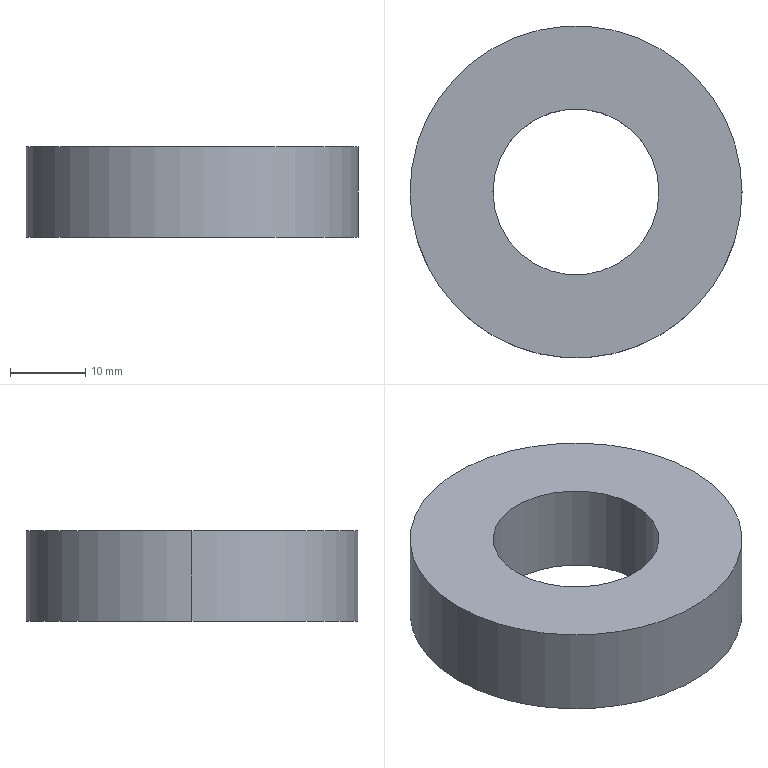Part | STEP file | 6022ZZ deep groove ball bearing MISUMI 62 | 1 solid | 6 faces | box 44 x 44 x 12 mm | volume 13685 mm3 | cylinder 4 | plane 2 | commonest cylinder face diameters 22 x2 44 x2
STEP:
#1=CARTESIAN_POINT('',(-11.,0.,6.));
#2=VERTEX_POINT('',#1);
#3=CARTESIAN_POINT('',(11.,0.,6.));
#4=VERTEX_POINT('',#3);
#5=CARTESIAN_POINT('',(0.,0.,6.));
#6=DIRECTION('',(0.,0.,1.));
#7=DIRECTION('',(1.,0.,0.));
#8=AXIS2_PLACEMENT_3D('',#5,#6,#7);
#9=CIRCLE('',#8,11.);
#10=EDGE_CURVE('',#2,#4,#9,.T.);
#11=ORIENTED_EDGE('',*,*,#10,.T.);
#12=CARTESIAN_POINT('',(11.,0.,-6.));
#13=VERTEX_POINT('',#12);
#14=CARTESIAN_POINT('',(11.,0.,6.));
#15=DIRECTION('',(0.,0.,-1.));
#16=VECTOR('',#15,1000.);
#17=LINE('',#14,#16);
#18=EDGE_CURVE('',#4,#13,#17,.T.);
#19=ORIENTED_EDGE('',*,*,#18,.T.);
#20=CARTESIAN_POINT('',(-11.,0.,-6.));
#21=VERTEX_POINT('',#20);
#22=CARTESIAN_POINT('',(0.,0.,-6.));
#23=DIRECTION('',(0.,0.,1.));
#24=DIRECTION('',(1.,0.,0.));
#25=AXIS2_PLACEMENT_3D('',#22,#23,#24);
#26=CIRCLE('',#25,11.);
#27=EDGE_CURVE('',#21,#13,#26,.T.);
#28=ORIENTED_EDGE('',*,*,#27,.F.);
#29=CARTESIAN_POINT('',(-11.,0.,6.));
#30=DIRECTION('',(0.,0.,-1.));
#31=VECTOR('',#30,1000.);
#32=LINE('',#29,#31);
#33=EDGE_CURVE('',#2,#21,#32,.T.);
#34=ORIENTED_EDGE('',*,*,#33,.F.);
#35=EDGE_LOOP('',(#11,#19,#28,#34));
#36=FACE_OUTER_BOUND('',#35,.T.);
#37=CARTESIAN_POINT('',(0.,0.,6.));
#38=DIRECTION('',(0.,0.,-1.));
#39=DIRECTION('',(-1.,0.,0.));
#40=AXIS2_PLACEMENT_3D('',#37,#38,#39);
#41=CYLINDRICAL_SURFACE('',#40,11.);
#42=ADVANCED_FACE('',(#36),#41,.F.);
#43=CARTESIAN_POINT('',(22.,0.,6.));
#44=VERTEX_POINT('',#43);
#45=CARTESIAN_POINT('',(-22.,0.,6.));
#46=VERTEX_POINT('',#45);
#47=CARTESIAN_POINT('',(0.,0.,6.));
#48=DIRECTION('',(0.,0.,1.));
#49=DIRECTION('',(1.,0.,0.));
#50=AXIS2_PLACEMENT_3D('',#47,#48,#49);
#51=CIRCLE('',#50,22.);
#52=EDGE_CURVE('',#44,#46,#51,.T.);
#53=ORIENTED_EDGE('',*,*,#52,.F.);
#54=CARTESIAN_POINT('',(22.,0.,-6.));
#55=VERTEX_POINT('',#54);
#56=CARTESIAN_POINT('',(22.,0.,6.));
#57=DIRECTION('',(0.,0.,-1.));
#58=VECTOR('',#57,1000.);
#59=LINE('',#56,#58);
#60=EDGE_CURVE('',#44,#55,#59,.T.);
#61=ORIENTED_EDGE('',*,*,#60,.T.);
#62=CARTESIAN_POINT('',(-22.,0.,-6.));
#63=VERTEX_POINT('',#62);
#64=CARTESIAN_POINT('',(0.,0.,-6.));
#65=DIRECTION('',(0.,0.,1.));
#66=DIRECTION('',(1.,0.,0.));
#67=AXIS2_PLACEMENT_3D('',#64,#65,#66);
#68=CIRCLE('',#67,22.);
#69=EDGE_CURVE('',#55,#63,#68,.T.);
#70=ORIENTED_EDGE('',*,*,#69,.T.);
#71=CARTESIAN_POINT('',(-22.,0.,6.));
#72=DIRECTION('',(0.,0.,-1.));
#73=VECTOR('',#72,1000.);
#74=LINE('',#71,#73);
#75=EDGE_CURVE('',#46,#63,#74,.T.);
#76=ORIENTED_EDGE('',*,*,#75,.F.);
#77=EDGE_LOOP('',(#53,#61,#70,#76));
#78=FACE_OUTER_BOUND('',#77,.T.);
#79=CARTESIAN_POINT('',(0.,0.,6.));
#80=DIRECTION('',(0.,0.,-1.));
#81=DIRECTION('',(-1.,0.,0.));
#82=AXIS2_PLACEMENT_3D('',#79,#80,#81);
#83=CYLINDRICAL_SURFACE('',#82,22.);
#84=ADVANCED_FACE('',(#78),#83,.T.);
#85=CARTESIAN_POINT('',(0.,0.,6.));
#86=DIRECTION('',(0.,0.,1.));
#87=DIRECTION('',(1.,0.,0.));
#88=AXIS2_PLACEMENT_3D('',#85,#86,#87);
#89=CIRCLE('',#88,22.);
#90=EDGE_CURVE('',#46,#44,#89,.T.);
#91=ORIENTED_EDGE('',*,*,#90,.T.);
#92=ORIENTED_EDGE('',*,*,#52,.T.);
#93=EDGE_LOOP('',(#91,#92));
#94=FACE_OUTER_BOUND('',#93,.T.);
#95=ORIENTED_EDGE('',*,*,#10,.F.);
#96=CARTESIAN_POINT('',(0.,0.,6.));
#97=DIRECTION('',(0.,0.,1.));
#98=DIRECTION('',(1.,0.,0.));
#99=AXIS2_PLACEMENT_3D('',#96,#97,#98);
#100=CIRCLE('',#99,11.);
#101=EDGE_CURVE('',#4,#2,#100,.T.);
#102=ORIENTED_EDGE('',*,*,#101,.F.);
#103=EDGE_LOOP('',(#95,#102));
#104=FACE_BOUND('',#103,.T.);
#105=CARTESIAN_POINT('',(0.,0.,6.));
#106=DIRECTION('',(0.,0.,1.));
#107=DIRECTION('',(1.,0.,0.));
#108=AXIS2_PLACEMENT_3D('',#105,#106,#107);
#109=PLANE('',#108);
#110=ADVANCED_FACE('',(#94,#104),#109,.T.);
#111=CARTESIAN_POINT('',(0.,0.,-6.));
#112=DIRECTION('',(0.,0.,1.));
#113=DIRECTION('',(1.,0.,0.));
#114=AXIS2_PLACEMENT_3D('',#111,#112,#113);
#115=CIRCLE('',#114,22.);
#116=EDGE_CURVE('',#63,#55,#115,.T.);
#117=ORIENTED_EDGE('',*,*,#116,.F.);
#118=ORIENTED_EDGE('',*,*,#69,.F.);
#119=EDGE_LOOP('',(#117,#118));
#120=FACE_OUTER_BOUND('',#119,.T.);
#121=ORIENTED_EDGE('',*,*,#27,.T.);
#122=CARTESIAN_POINT('',(0.,0.,-6.));
#123=DIRECTION('',(0.,0.,1.));
#124=DIRECTION('',(1.,0.,0.));
#125=AXIS2_PLACEMENT_3D('',#122,#123,#124);
#126=CIRCLE('',#125,11.);
#127=EDGE_CURVE('',#13,#21,#126,.T.);
#128=ORIENTED_EDGE('',*,*,#127,.T.);
#129=EDGE_LOOP('',(#121,#128));
#130=FACE_BOUND('',#129,.T.);
#131=CARTESIAN_POINT('',(0.,0.,-6.));
#132=DIRECTION('',(0.,0.,1.));
#133=DIRECTION('',(1.,0.,0.));
#134=AXIS2_PLACEMENT_3D('',#131,#132,#133);
#135=PLANE('',#134);
#136=ADVANCED_FACE('',(#120,#130),#135,.F.);
#137=ORIENTED_EDGE('',*,*,#60,.F.);
#138=ORIENTED_EDGE('',*,*,#90,.F.);
#139=ORIENTED_EDGE('',*,*,#75,.T.);
#140=ORIENTED_EDGE('',*,*,#116,.T.);
#141=EDGE_LOOP('',(#137,#138,#139,#140));
#142=FACE_OUTER_BOUND('',#141,.T.);
#143=CARTESIAN_POINT('',(0.,0.,6.));
#144=DIRECTION('',(0.,0.,-1.));
#145=DIRECTION('',(-1.,0.,0.));
#146=AXIS2_PLACEMENT_3D('',#143,#144,#145);
#147=CYLINDRICAL_SURFACE('',#146,22.);
#148=ADVANCED_FACE('',(#142),#147,.T.);
#149=ORIENTED_EDGE('',*,*,#18,.F.);
#150=ORIENTED_EDGE('',*,*,#101,.T.);
#151=ORIENTED_EDGE('',*,*,#33,.T.);
#152=ORIENTED_EDGE('',*,*,#127,.F.);
#153=EDGE_LOOP('',(#149,#150,#151,#152));
#154=FACE_OUTER_BOUND('',#153,.T.);
#155=CARTESIAN_POINT('',(0.,0.,6.));
#156=DIRECTION('',(0.,0.,-1.));
#157=DIRECTION('',(-1.,0.,0.));
#158=AXIS2_PLACEMENT_3D('',#155,#156,#157);
#159=CYLINDRICAL_SURFACE('',#158,11.);
#160=ADVANCED_FACE('',(#154),#159,.F.);
#161=CLOSED_SHELL('',(#42,#84,#110,#136,#148,#160));
#162=MANIFOLD_SOLID_BREP('',#161);
#163=CARTESIAN_POINT('',(0.,0.,0.));
#164=DIRECTION('',(0.,0.,1.));
#165=DIRECTION('',(1.,0.,0.));
#166=AXIS2_PLACEMENT_3D('',#163,#164,#165);
#167=(LENGTH_UNIT()NAMED_UNIT(*)SI_UNIT(.MILLI.,.METRE.));
#168=UNCERTAINTY_MEASURE_WITH_UNIT(LENGTH_MEASURE(0.00001),#167,'','');
#169=(NAMED_UNIT(*)PLANE_ANGLE_UNIT()SI_UNIT($,.RADIAN.));
#170=(NAMED_UNIT(*)SI_UNIT($,.STERADIAN.)SOLID_ANGLE_UNIT());
#171=(GEOMETRIC_REPRESENTATION_CONTEXT(3)GLOBAL_UNCERTAINTY_ASSIGNED_CONTEXT((#168))GLOBAL_UNIT_ASSIGNED_CONTEXT((#167,#169,#170))REPRESENTATION_CONTEXT('',''));
#172=ADVANCED_BREP_SHAPE_REPRESENTATION('',(#162,#166),#171);